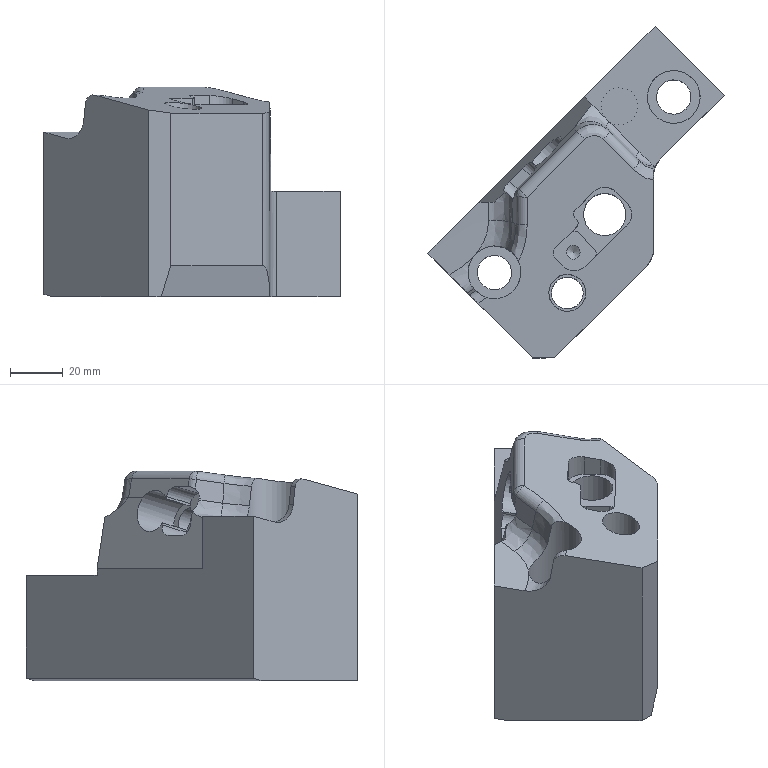Part | STEP file | gslz 2016.10.28-13_id366_x_t | 1 solid | 89 faces | box 112.236 x 125.671 x 79.488 mm | volume 334132 mm3 | plane 33 | cylinder 32 | spline 19 | cone 2 | other 2 | sphere 1 | commonest cylinder face diameters 12 x5 4 x4 8 x4 7.5 x3 5.2 x2 13 x2